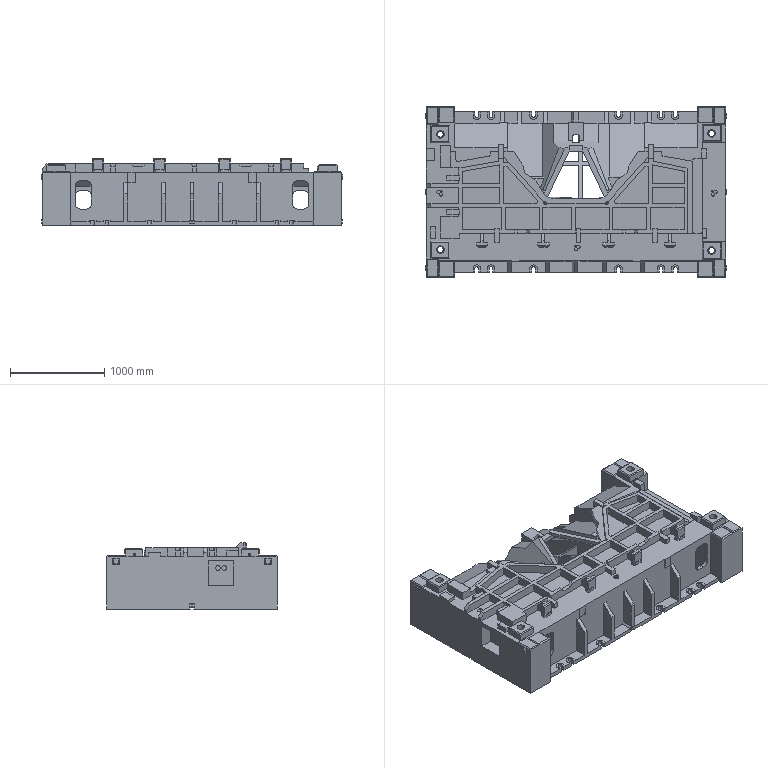Part | NX | features solid 2 | 1 solid | 1397 faces | box 3190 x 1800 x 700 mm | volume 916882021 mm3 | plane 1082 | cylinder 244 | spline 69 | cone 2 | commonest cylinder face diameters 100 x168 40 x16 80 x16 50 x11 20 x9 10 x7